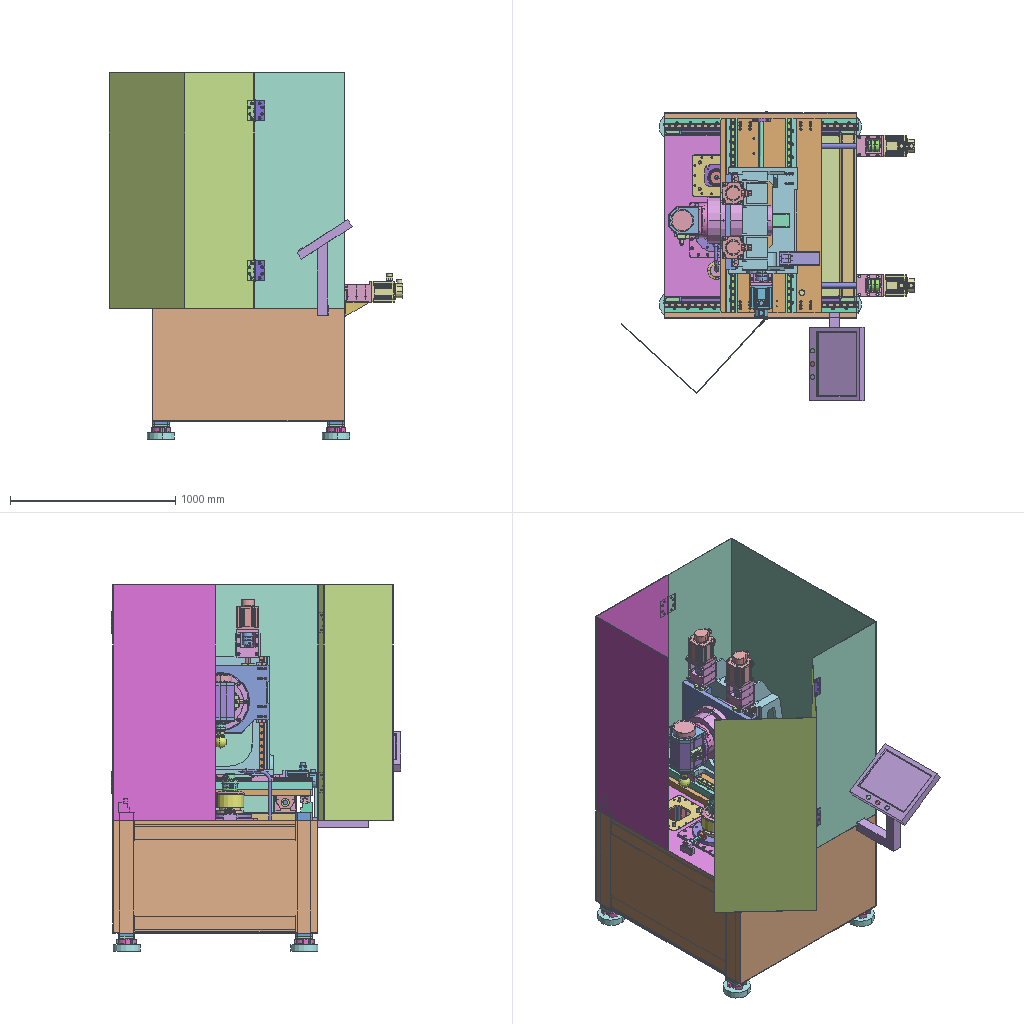Assembly | SolidWorks | 96 different items | 189 placed | box 1776 x 1752 x 2219 mm
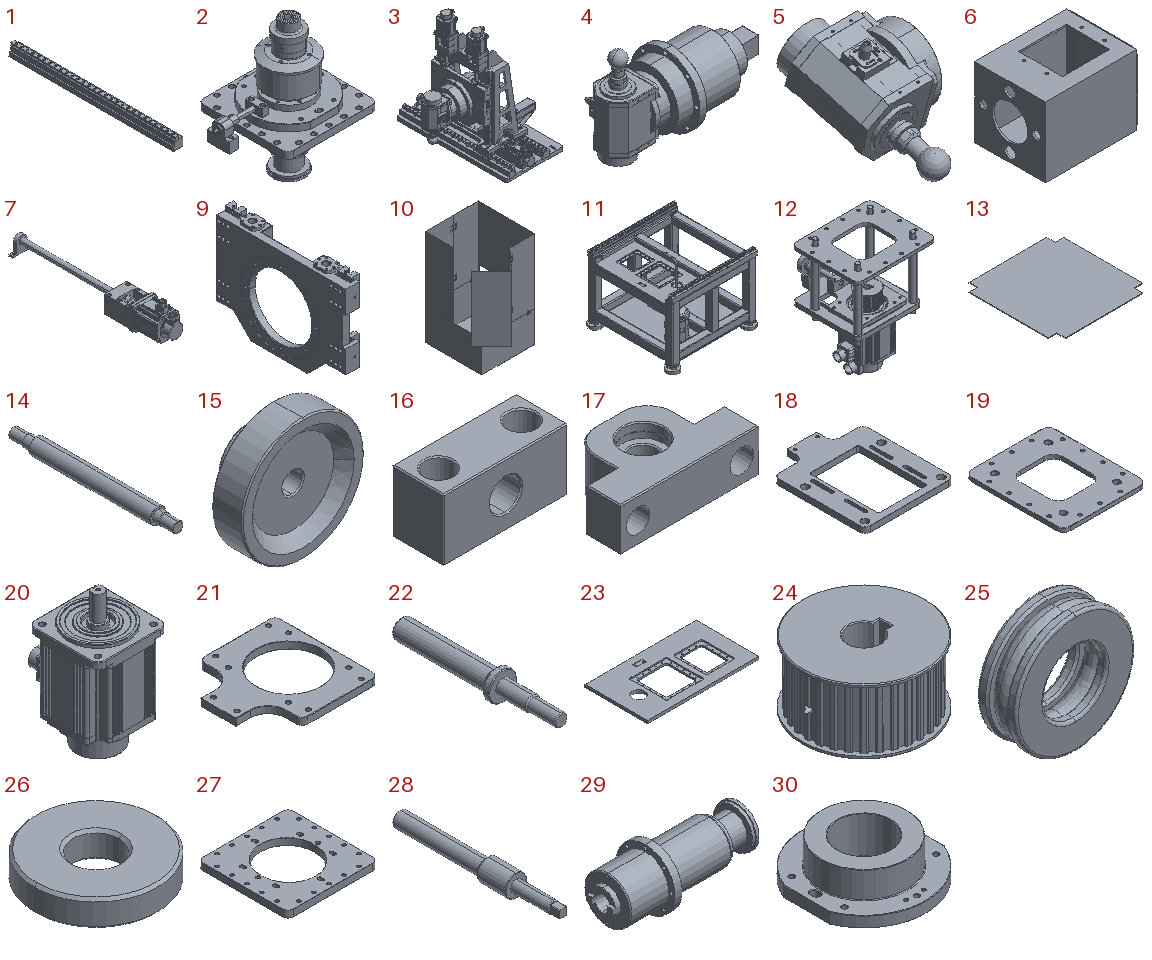Parts list (item | name | quantity | parent item | size | volume | features):
1 | (subassembly) | x2 | in 11 | 70 x 1176 x 83 mm | 4869056 mm3 | -
2 | (subassembly) | x1 | - | 435.5 x 330 x 510 mm | 9332980 mm3 | -
3 | (subassembly) | x1 | - | - | 102091966 mm3 | -
4 | (subassembly) | x1 | in 3 | 732.6 x 340 x 450.98 mm | 29819658 mm3 | -
5 | (subassembly) | x1 | in 4 | 237.6 x 446.584 x 263.499 mm | 8299618 mm3 | -
6 | (subassembly) | x1 | in 4 | 105 x 80 x 80 mm | 78423 mm3 | -
7 | (subassembly) | x2 | - | 130 x 914.5 x 177.75 mm | 425497 mm3 | -
8 | (subassembly) | x1 | in 3 | - | - | -
9 | (subassembly) | x1 | in 3 | 82 x 575 x 437.9 mm | 6520185 mm3 | -
10 | (subassembly) | x1 | - | 1424 x 1708 x 2109 mm | 23017805 mm3 | features CompositeCurve 2
11 | (subassembly) | x1 | - | 1225 x 1241 x 1104 mm | 76419257 mm3 | -
12 | (subassembly) | x1 | - | 295 x 346 x 412 mm | 272069 mm3 | -
13 | - | x1 | in 11 | 1160 x 1176 x 8 mm | 10560480 mm3 | features BaseBody 1
14 | - | x4 | in 12 | 25 x 260.5 x 25 mm | 109382 mm3 | features BaseBody 1
15 | - | x1 | in 12 | 60 x 29 x 60 mm | 41614 mm3 | features BaseBody 1
16 | - | x1 | in 12 | 60 x 25 x 30 mm | 34275 mm3 | features BaseBody 1
17 | - | x1 | in 12 | 80 x 47 x 25 mm | 53700 mm3 | features BaseBody 1
18 | - | x1 | in 12 | 240 x 290 x 16 mm | 561839 mm3 | features BaseBody 1
19 | - | x1 | in 12 | 250 x 295 x 12 mm | 640437 mm3 | features BaseBody 1
20 | - | x2 | in 3, 12 | - | - | features RefSurface 1
21 | - | x1 | in 12 | 185 x 176 x 12 mm | 199285 mm3 | features BaseBody 1
22 | - | x1 | in 12 | 23 x 131 x 23 mm | 22576 mm3 | features BaseBody 1
23 | - | x1 | in 11 | 976 x 550 x 25 mm | 9505923 mm3 | features BaseBody 1
24 | - | x1 | in 12 | 85.12 x 85.12 x 55 mm | 217728 mm3 | features BaseBody 1
25 | - | x4 | in 2, 12 | 23 x 7.5 x 23 mm | 1948 mm3 | features BaseBody 1
26 | - | x2 | in 2 | 28 x 28 x 6 mm | 3096 mm3 | features BaseBody 1
27 | - | x1 | in 2 | 330 x 330 x 25 mm | 1816926 mm3 | features BaseBody 1
28 | - | x1 | in 2 | 23 x 175 x 23 mm | 36998 mm3 | features BaseBody 1
29 | - | x1 | in 2 | 416 x 165 x 165 mm | 4108443 mm3 | features BaseBody 1
30 | - | x1 | in 2 | 260 x 280 x 85 mm | 2297762 mm3 | features BaseBody 1
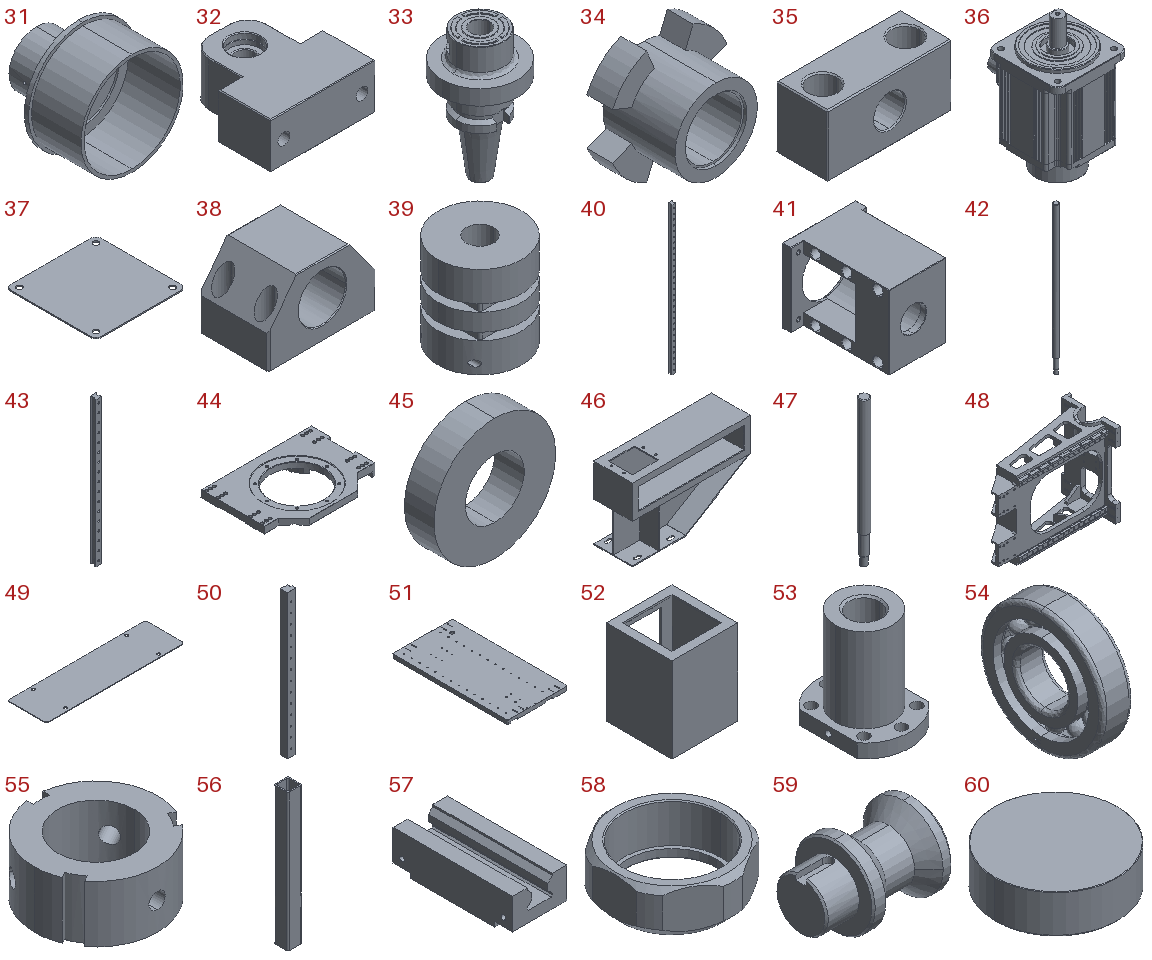31 | - | x1 | in 2 | 180 x 159.011 x 180 mm | 532687 mm3 | features BaseBody 4
32 | - | x1 | in 2 | 80 x 80 x 35 mm | 146595 mm3 | features BaseBody 1
33 | - | x1 | in 2 | 100 x 100 x 169.5 mm | 348963 mm3 | features BaseBody 1
34 | - | x4 | in 11 | 111.243 x 75 x 111.243 mm | 319266 mm3 | features BaseBody 1
35 | - | x1 | in 2 | 60 x 25 x 30 mm | 34266 mm3 | features BaseBody 1
36 | - | x2 | in 3 | 130 x 176.14 x 238.5 mm | 2461852 mm3 | features BaseBody 1
37 | - | x1 | in 6 | 80 x 80 x 1 mm | 6300 mm3 | features BaseBody 1
38 | - | x3 | in 3 | 115 x 73 x 75 mm | 354345 mm3 | features BaseBody 1
39 | - | x3 | in 3 | 68 x 68 x 74 mm | 205808 mm3 | features BaseBody 1
40 | - | x2 | in 3 | 28 x 28 x 1176 mm | 695129 mm3 | features BaseBody 1
41 | - | x3 | in 3 | 130 x 167 x 130 mm | 1161837 mm3 | features BaseBody 1
42 | - | x1 | in 3 | 32 x 32 x 950.5 mm | 728674 mm3 | features BaseBody 1, MoveFace 1
43 | - | x2 | in 3 | 28 x 28 x 680 mm | 401283 mm3 | features BaseBody 1
44 | - | x1 | in 9 | 575 x 410 x 82 mm | 5326767 mm3 | features BaseBody 1
45 | - | x4 | in 11 | 165 x 40 x 165 mm | 654237 mm3 | features BaseBody 1
46 | - | x1 | in 3 | 245 x 80 x 151 mm | 206222 mm3 | features BaseBody 2
47 | - | x2 | in 3 | 32 x 32 x 484 mm | 353493 mm3 | features BaseBody 1
48 | - | x1 | in 3 | 881 x 420 x 640 mm | 19459611 mm3 | features BaseBody 1
49 | - | x1 | in 3 | 245 x 69 x 1 mm | 16805 mm3 | features BaseBody 1
50 | - | x2 | in 3 | 70 x 60 x 1176 mm | 4173927 mm3 | features BaseBody 1
51 | - | x1 | in 3 | 610 x 1176 x 40 mm | 25279408 mm3 | features HoleWzd 4, ICE 2, BaseBody 1, MoveFace 1
52 | - | x1 | in 6 | 80 x 80 x 104 mm | 72123 mm3 | features BaseBody 1
53 | - | x5 | in 3, 9 | 62 x 80 x 85 mm | 142057 mm3 | features BaseBody 1
54 | - | x9 | in 3 | 15 x 62 x 62 mm | 27962 mm3 | features BaseBody 14
55 | - | x3 | in 3 | 38 x 37.835 x 18 mm | 11538 mm3 | features BaseBody 1
56 | - | x6 | in 11 | 100 x 100 x 976 mm | 2843183 mm3 | features BaseBody 1
57 | - | x8 | in 3, 9 | 60 x 143.8 x 39 mm | 227326 mm3 | features BaseBody 1
58 | - | x1 | in 5 | 56 x 60 x 23 mm | 20223 mm3 | features BaseBody 1
59 | - | x1 | in 5 | 56 x 39 x 39 mm | 37628 mm3 | features BaseBody 1
60 | - | x1 | in 5 | 140 x 140 x 45 mm | 200339 mm3 | features BaseBody 1
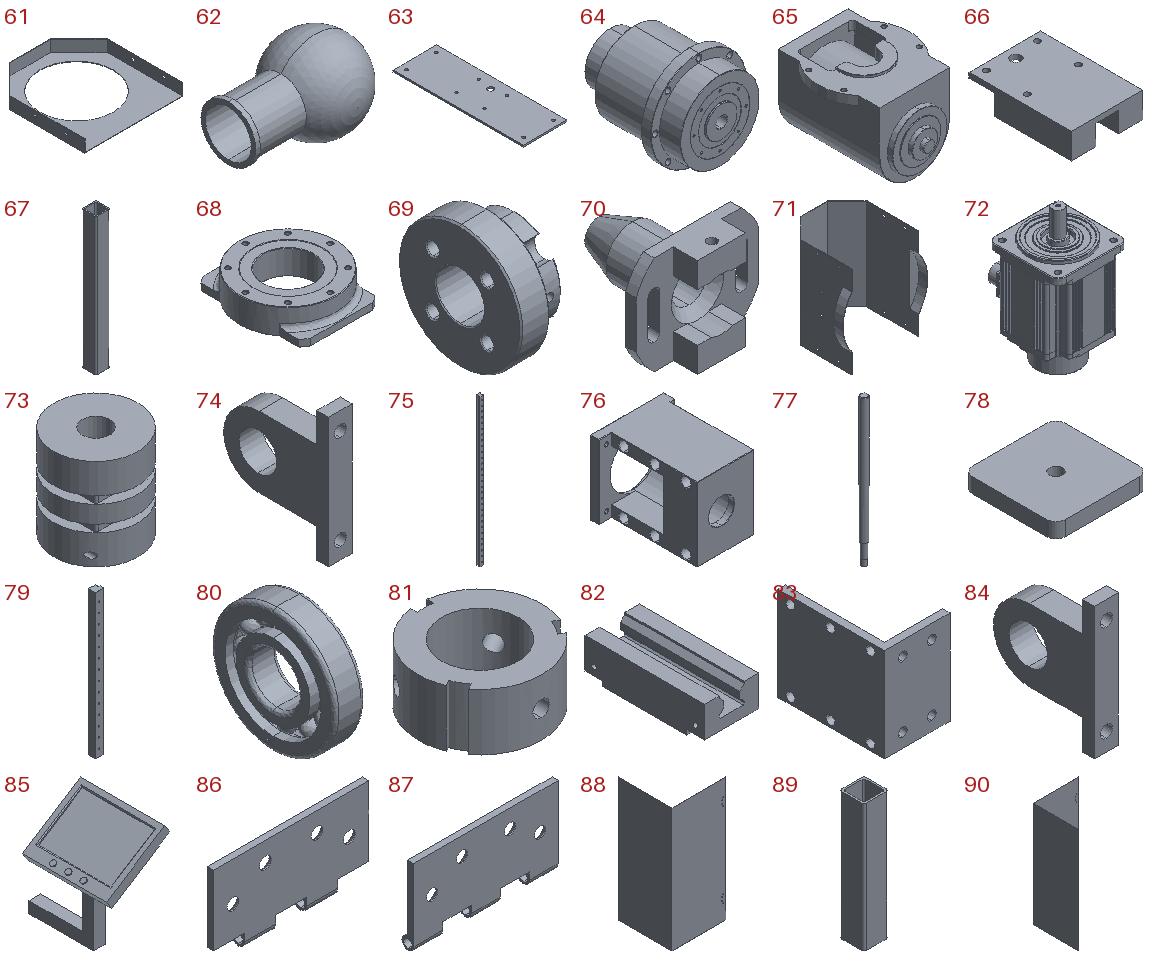61 | - | x2 | in 5 | 172 x 182 x 21 mm | 25333 mm3 | features BaseBody 1
62 | - | x1 | in 5 | 109.98 x 72.246 x 72.246 mm | 221727 mm3 | features BaseBody 1, Revolution 1
63 | - | x1 | in 5 | 78 x 231 x 3 mm | 53417 mm3 | features BaseBody 1
64 | - | x1 | in 4 | 340 x 396 x 340 mm | 21441939 mm3 | features BaseBody 1, ICE 1
65 | - | x1 | in 5 | 210 x 300 x 185.1 mm | 5982188 mm3 | features BaseBody 1
66 | - | x1 | in 5 | 70 x 100 x 25 mm | 106773 mm3 | features BaseBody 1
67 | - | x4 | in 11 | 100 x 100 x 960 mm | 2796573 mm3 | features BaseBody 1
68 | - | x1 | in 5 | 210 x 234 x 55.5 mm | 1439781 mm3 | features BaseBody 1
69 | - | x1 | in 5 | 30 x 64 x 64 mm | 51096 mm3 | features BaseBody 1
70 | - | x1 | in 5 | 56 x 56 x 45 mm | 24024 mm3 | features BaseBody 1
71 | - | x1 | in 5 | 214 x 180 x 230 mm | 111689 mm3 | features BaseBody 1
72 | - | x2 | in 7 | - | - | features RefSurface 1
73 | - | x2 | in 7 | 68 x 68 x 74 mm | 205808 mm3 | features BaseBody 1
74 | - | x2 | in 7 | 20 x 89 x 110 mm | 91419 mm3 | features MoveFace 4, BaseBody 1, DelFace 1, HoleWzd 1, ICE 1, Split 1
75 | - | x2 | in 1 | 28 x 28 x 1176 mm | 695129 mm3 | features BaseBody 1
76 | - | x2 | in 7 | 130 x 167 x 130 mm | 1168663 mm3 | features ICE 2, BaseBody 1, BossThin 1, DelFace 1, DeleteBody 1
77 | - | x2 | in 7 | 32 x 32 x 664 mm | 498257 mm3 | features BaseBody 1
78 | - | x4 | in 11 | 100 x 100 x 16 mm | 156164 mm3 | features BaseBody 1
79 | - | x2 | in 1 | 70 x 60 x 1176 mm | 4173927 mm3 | features BaseBody 1
80 | - | x6 | in 7 | 15 x 62 x 62 mm | 27962 mm3 | features BaseBody 14
81 | - | x2 | in 7 | 38 x 37.835 x 18 mm | 11538 mm3 | features BaseBody 1
82 | - | x4 | - | 60 x 143.8 x 39 mm | 227326 mm3 | features BaseBody 1, Split 1
83 | - | x2 | - | 90 x 146.4 x 128.8 mm | 334625 mm3 | features BaseBody 1, HoleWzd 1
84 | - | x1 | in 3 | 20 x 84 x 110 mm | 85419 mm3 | features MoveFace 6, BaseBody 1, DelFace 1, HoleWzd 1, ICE 1, Split 1
85 | - | x1 | - | 334.254 x 534.204 x 579.086 mm | 9689433 mm3 | features ICE 2, BossThin 1, Chamfer 1, Extrusion 1, MoveFace 1, Split 1
86 | - | x4 | in 10 | 120 x 10 x 65 mm | 32275 mm3 | features BaseBody 1
87 | - | x4 | in 10 | 120 x 10 x 65 mm | 33485 mm3 | features BaseBody 1
88 | - | x1 | in 10 | 620 x 620 x 1428 mm | 3533218 mm3 | features BaseBody 1
89 | - | x2 | in 11 | 100 x 100 x 520 mm | 1514811 mm3 | features BaseBody 1
90 | - | x1 | in 10 | 620 x 621.122 x 1428 mm | 3536422 mm3 | features BaseBody 1
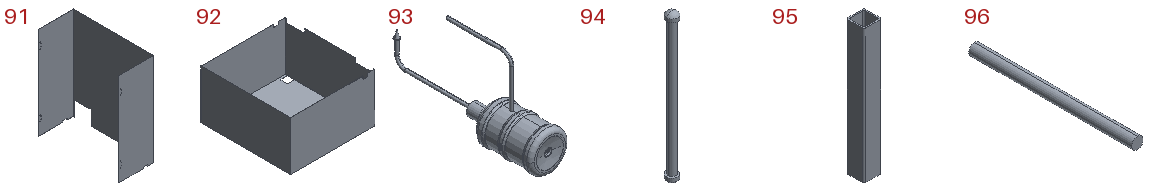91 | - | x1 | in 10 | 544 x 1240 x 1428 mm | 6405923 mm3 | features BaseBody 1
92 | - | x1 | in 10 | 1164 x 1240 x 681 mm | 9260336 mm3 | features BaseBody 1
93 | - | x1 | in 11 | 245.999 x 983.22 x 550.042 mm | 1897032 mm3 | features Split 3, Revolution 2, Sweep 2, BaseBody 1, DelFace 1, Fillet 1, ICE 1
94 | - | x4 | in 10 | 10 x 10 x 132 mm | 4717 mm3 | features BaseBody 1
95 | - | x4 | in 11 | 100 x 100 x 750 mm | 2184823 mm3 | features BaseBody 1
96 | - | x4 | in 11 | 16 x 230 x 16 mm | 46244 mm3 | features BaseBody 1
Mates (type | each side: item.copy, entity, surface, feature):
In the top assembly
Coincident | 75.1 face plane Input1 | 82.1 face plane Input1 | 2 times
Coincident | 75.2 face plane Input1 | 82.2 face plane Input1 | 2 times
Coincident | 82.1 face plane Input1 | 82.2 face plane Input1
Coincident | 51.1 face plane Input1 | 82.1 face plane Input1
DistanceDim | 51.1 face plane Input1 | 79.1 face plane Input1
Coincident | 75.1 face plane Input1 | 82.3 face plane Input1 | 2 times
Coincident | 75.2 face plane Input1 | 82.4 face plane Input1 | 2 times
DistanceDim | 82.4 face cylinder Input1 | 82.2 face cylinder Input1
Coincident | 82.3 face plane Input1 | 82.4 face plane Input1
Coincident | 50.1 face plane Input1 | 82.2 face plane Input1
Concentric | 53.1 face cylinder Input1 | 77.1 face cylinder Input1
Parallel | 56.1 face plane Input1 | 76.1 face plane Input1
Coincident | 76.1 face plane Input1 | 83.1 face plane Input1
Concentric | 76.1 face cylinder Input1 | 83.1 face cylinder Input1 | 2 times
Coincident | 56.1 face plane Input1 | 83.1 face plane Input1
Coincident | 76.2 face plane Input1 | 83.2 face plane Input1
Concentric | 76.2 face cylinder Input1 | 83.2 face cylinder Input1 | 2 times
Coincident | 56.1 face plane Input1 | 83.2 face plane Input1
Coincident | 95.1 face plane Input1 | 83.2 face plane Input1
Concentric | 38.1 face cylinder Input1 | 53.2 face cylinder Input1 | 2 times
Coincident | 38.1 face plane Input1 | 53.2 face plane Input1
Concentric | 77.2 face cylinder Input1 | 53.2 face cylinder Input1
Coincident | 51.1 face plane Input1 | 38.1 face plane Input1
Coincident | 38.2 face plane Input1 | 38.1 face plane Input1
In subassembly 11
Coincident | 67.1 face plane Input1 | 79.2 face plane Input1 | 2 times
Coincident | 95.2 face plane Input1 | 79.2 face plane Input1
Coincident | 95.3 face plane Input1 | 79.3 face plane Input1
Coincident | 67.2 face plane Input1 | 79.3 face plane Input1 | 2 times
Coincident | 13.1 face plane Input1 | 93.1 plane
Concentric | 23.1 face cylinder Input1 | 93.1 face cylinder Sweep 1
In subassembly 3
Coincident | 51.2 face plane Input1 | 3.1 face
Concentric | 51.2 face cylinder Sizemm Dowel PinHole 1 | 3.1 face | 2 times
Coincident | 51.2 face plane Input1 | 38.1 face plane Input1
Concentric | 51.2 face cylinder Sizemm Dowel PinHole 1 | 38.1 face cylinder Input1 | 2 times
Concentric | 38.1 face cylinder Input1 | 53.3 face cylinder Input1 | 2 times
Coincident | 38.1 face plane Input1 | 53.3 face plane Input1
Concentric | 42.1 face cylinder Input1 | 84.1 face cylinder Input1
Parallel | 51.2 face plane Input1 | 84.1 face plane Input1
Coincident | 51.2 face plane Input1 | 84.1 face plane Input1
Concentric | 53.4 face cylinder Input1 | 47.1 face cylinder Input1
Concentric | 53.5 face cylinder Input1 | 47.2 face cylinder Input1
Concentric | 44.1 face cylinder Input1 | 64.1 face cylinder Input1 | 2 times
Coincident | 44.1 face plane Input1 | 64.1 face plane Input1
In subassembly 4
Concentric | 68.1 face cylinder Input1 | 64.2 face cylinder Input1
Concentric | 64.2 face cylinder Input1 | 52.1 face cylinder Input1
Coincident | 64.2 face plane Input1 | 52.1 face plane Input1
In subassembly 7
Concentric | 74.1 face cylinder Input1 | 77.3 face cylinder Input1
Coincident | 74.1 face plane Input1 | 77.3 face plane Input1
Parallel | 74.1 face plane Input1 | 76.3 face plane Input1
In subassembly 10
Concentric | 91.1 face cylinder Input3 | 86.1 face cylinder Input1 | 2 times
Concentric | 90.1 face cylinder Input3 | 87.1 face cylinder Input1 | 2 times
Concentric | 87.1 face cylinder Input1 | 86.1 face cylinder Input1
Concentric | 87.1 face cylinder Input1 | 94.1 face cylinder Input1
Coincident | 87.1 face plane Input1 | 94.1 face plane Input1
Concentric | 91.1 face cylinder Input3 | 86.2 edge
Concentric | 91.1 face cylinder Input3 | 86.2 face cylinder Input1
Concentric | 90.1 face cylinder Input3 | 87.2 face cylinder Input1 | 2 times
Concentric | 87.2 face cylinder Input1 | 86.2 face cylinder Input1
Concentric | 87.2 face cylinder Input1 | 94.2 face cylinder Input1
Coincident | 87.2 face plane Input1 | 94.2 face plane Input1
Coincident | 91.1 face plane Input3 | 86.1 face plane Input1
Coincident | 90.1 face plane Input3 | 87.1 face plane Input1
Coincident | 87.1 face plane Input1 | 86.1 face plane Input1
Concentric | 91.1 face cylinder Input3 | 87.3 face cylinder Input1 | 2 times
Concentric | 88.1 face cylinder Input3 | 86.3 face cylinder Input1 | 2 times
Concentric | 91.1 face cylinder Input3 | 87.4 face cylinder Input1 | 2 times
Concentric | 88.1 face cylinder Input3 | 86.4 face cylinder Input1 | 2 times
Coincident | 91.1 face plane Input3 | 87.4 face plane Input1
Coincident | 88.1 face plane Input3 | 86.4 face plane Input1
Concentric | 87.4 face cylinder Input1 | 86.4 face cylinder Input1
Coincident | 87.4 face plane Input1 | 86.4 face plane Input1
Concentric | 87.4 face cylinder Input1 | 94.3 face cylinder Input1
Coincident | 87.4 face plane Input1 | 94.3 edge
Concentric | 86.3 face cylinder Input1 | 94.4 face cylinder Input1
Concentric | 87.3 face cylinder Input1 | 94.4 face cylinder Input1
Parallel | 90.1 face plane Input3 | 92.1 face plane Input3